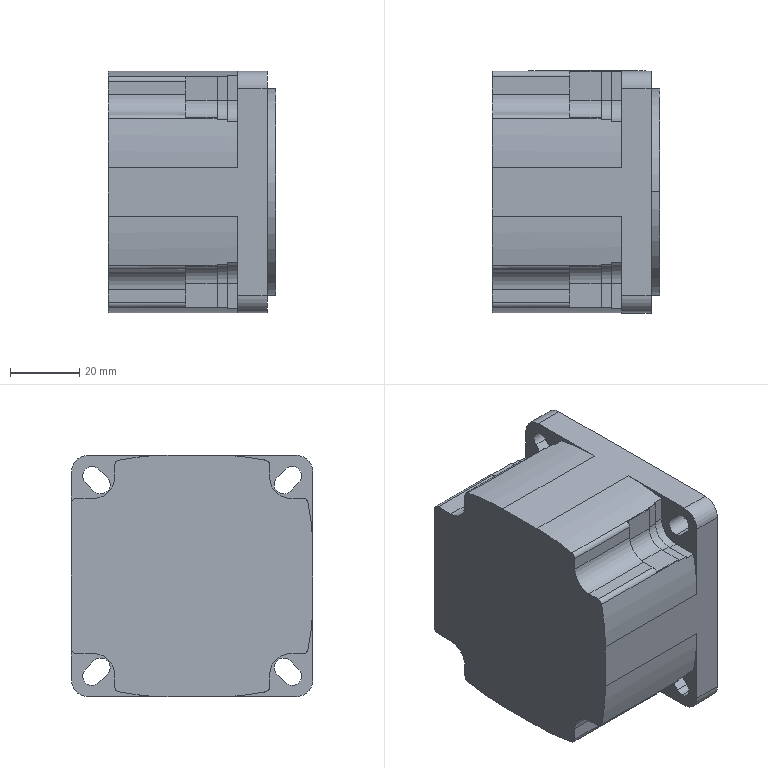Part | STEP file | HI_BMH070 Flansch | 1 solid | 164 faces | box 48.5 x 70.1 x 70 mm | volume 191060 mm3 | plane 93 | cylinder 65 | cone 6 | commonest cylinder face diameters 5.5 x12 12 x10 3 x8 10 x8 11 x6 140 x6